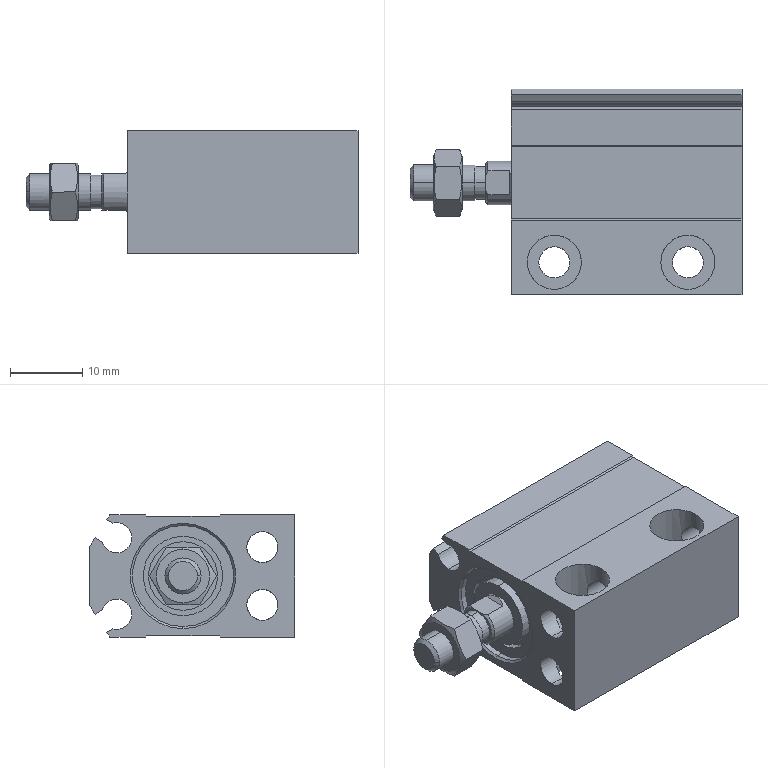Part | SolidWorks | features BaseBody 3 | 3 solids | 122 faces | box 46 x 28.5 x 17 mm | volume 11423 mm3 | cylinder 54 | plane 50 | cone 18 | commonest cylinder face diameters 4.3 x16 7.5 x8 4.134 x6 4.2 x6 6 x4 12 x4